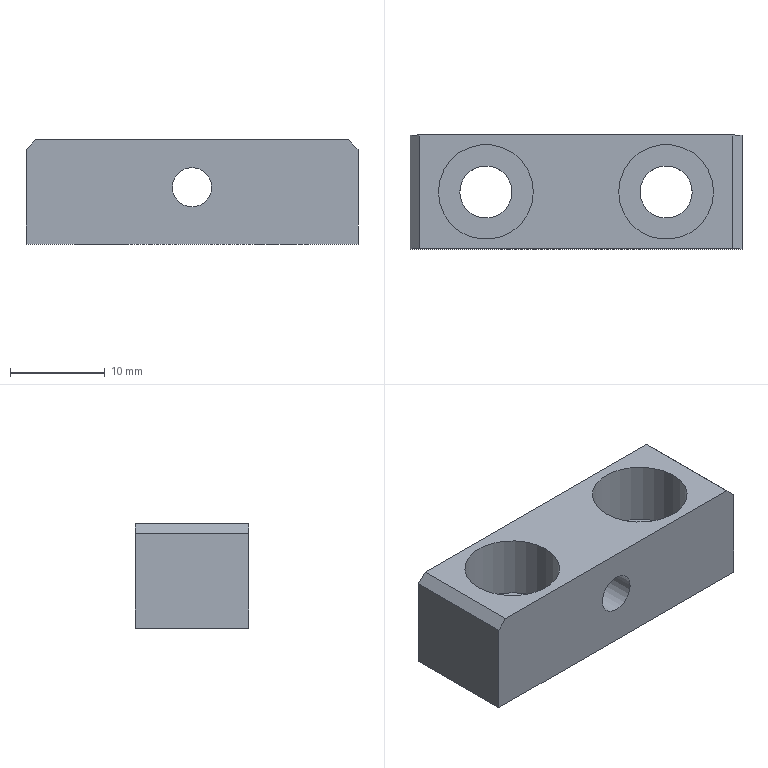Part | NX | features 5003_233_Adjusting screw block 2 | 1 solid | 15 faces | box 35 x 12 x 11 mm | volume 3190 mm3 | plane 10 | cylinder 5 | commonest cylinder face diameters 5.5 x2 10 x2 4.135 x1
STEP:
#1=CARTESIAN_POINT('',(9.775,118.5,-187.));
#2=VERTEX_POINT('',#1);
#3=CARTESIAN_POINT('',(9.775,118.5,-177.));
#4=VERTEX_POINT('',#3);
#5=CARTESIAN_POINT('',(9.775,118.5,-176.));
#6=DIRECTION('',(0.,0.,1.));
#7=VECTOR('',#6,1000.);
#8=LINE('',#5,#7);
#9=EDGE_CURVE('',#2,#4,#8,.T.);
#10=ORIENTED_EDGE('',*,*,#9,.T.);
#11=CARTESIAN_POINT('',(9.775,106.5,-177.));
#12=VERTEX_POINT('',#11);
#13=CARTESIAN_POINT('',(9.775,106.5,-177.));
#14=DIRECTION('',(0.,-1.,0.));
#15=VECTOR('',#14,1000.);
#16=LINE('',#13,#15);
#17=EDGE_CURVE('',#4,#12,#16,.T.);
#18=ORIENTED_EDGE('',*,*,#17,.T.);
#19=CARTESIAN_POINT('',(9.775,106.5,-187.));
#20=VERTEX_POINT('',#19);
#21=CARTESIAN_POINT('',(9.775,106.5,-176.));
#22=DIRECTION('',(0.,0.,1.));
#23=VECTOR('',#22,1000.);
#24=LINE('',#21,#23);
#25=EDGE_CURVE('',#20,#12,#24,.T.);
#26=ORIENTED_EDGE('',*,*,#25,.F.);
#27=CARTESIAN_POINT('',(9.775,106.5,-187.));
#28=DIRECTION('',(0.,1.,0.));
#29=VECTOR('',#28,1000.);
#30=LINE('',#27,#29);
#31=EDGE_CURVE('',#20,#2,#30,.T.);
#32=ORIENTED_EDGE('',*,*,#31,.T.);
#33=EDGE_LOOP('',(#10,#18,#26,#32));
#34=FACE_BOUND('',#33,.T.);
#35=CARTESIAN_POINT('',(9.775,106.5,-176.));
#36=DIRECTION('',(-1.,0.,0.));
#37=DIRECTION('',(0.,-1.,0.));
#38=AXIS2_PLACEMENT_3D('',#35,#36,#37);
#39=PLANE('',#38);
#40=ADVANCED_FACE('',(#34),#39,.F.);
#41=CARTESIAN_POINT('',(-22.225,112.5,-176.));
#42=VERTEX_POINT('',#41);
#43=CARTESIAN_POINT('',(-17.225,112.5,-176.));
#44=DIRECTION('',(0.,0.,1.));
#45=DIRECTION('',(-1.,0.,0.));
#46=AXIS2_PLACEMENT_3D('',#43,#44,#45);
#47=CIRCLE('',#46,5.);
#48=EDGE_CURVE('',#42,#42,#47,.T.);
#49=ORIENTED_EDGE('',*,*,#48,.F.);
#50=EDGE_LOOP('',(#49));
#51=FACE_BOUND('',#50,.T.);
#52=CARTESIAN_POINT('',(-3.225,112.5,-176.));
#53=VERTEX_POINT('',#52);
#54=CARTESIAN_POINT('',(1.775,112.5,-176.));
#55=DIRECTION('',(0.,0.,1.));
#56=DIRECTION('',(-1.,0.,0.));
#57=AXIS2_PLACEMENT_3D('',#54,#55,#56);
#58=CIRCLE('',#57,5.);
#59=EDGE_CURVE('',#53,#53,#58,.T.);
#60=ORIENTED_EDGE('',*,*,#59,.F.);
#61=EDGE_LOOP('',(#60));
#62=FACE_BOUND('',#61,.T.);
#63=CARTESIAN_POINT('',(8.775,106.5,-176.));
#64=VERTEX_POINT('',#63);
#65=CARTESIAN_POINT('',(-24.225,106.5,-176.));
#66=VERTEX_POINT('',#65);
#67=CARTESIAN_POINT('',(-25.225,106.5,-176.));
#68=DIRECTION('',(-1.,0.,0.));
#69=VECTOR('',#68,1000.);
#70=LINE('',#67,#69);
#71=EDGE_CURVE('',#64,#66,#70,.T.);
#72=ORIENTED_EDGE('',*,*,#71,.F.);
#73=CARTESIAN_POINT('',(8.775,118.5,-176.));
#74=VERTEX_POINT('',#73);
#75=CARTESIAN_POINT('',(8.775,106.5,-176.));
#76=DIRECTION('',(0.,1.,0.));
#77=VECTOR('',#76,1000.);
#78=LINE('',#75,#77);
#79=EDGE_CURVE('',#64,#74,#78,.T.);
#80=ORIENTED_EDGE('',*,*,#79,.T.);
#81=CARTESIAN_POINT('',(-24.225,118.5,-176.));
#82=VERTEX_POINT('',#81);
#83=CARTESIAN_POINT('',(-25.225,118.5,-176.));
#84=DIRECTION('',(-1.,0.,0.));
#85=VECTOR('',#84,1000.);
#86=LINE('',#83,#85);
#87=EDGE_CURVE('',#74,#82,#86,.T.);
#88=ORIENTED_EDGE('',*,*,#87,.T.);
#89=CARTESIAN_POINT('',(-24.225,106.5,-176.));
#90=DIRECTION('',(0.,-1.,0.));
#91=VECTOR('',#90,1000.);
#92=LINE('',#89,#91);
#93=EDGE_CURVE('',#82,#66,#92,.T.);
#94=ORIENTED_EDGE('',*,*,#93,.T.);
#95=EDGE_LOOP('',(#72,#80,#88,#94));
#96=FACE_BOUND('',#95,.T.);
#97=CARTESIAN_POINT('',(-25.225,106.5,-176.));
#98=DIRECTION('',(0.,0.,-1.));
#99=DIRECTION('',(1.,0.,0.));
#100=AXIS2_PLACEMENT_3D('',#97,#98,#99);
#101=PLANE('',#100);
#102=ADVANCED_FACE('',(#51,#62,#96),#101,.F.);
#103=CARTESIAN_POINT('',(-25.225,106.5,-177.));
#104=VERTEX_POINT('',#103);
#105=CARTESIAN_POINT('',(-25.225,106.5,-187.));
#106=VERTEX_POINT('',#105);
#107=CARTESIAN_POINT('',(-25.225,106.5,-176.));
#108=DIRECTION('',(0.,0.,-1.));
#109=VECTOR('',#108,1000.);
#110=LINE('',#107,#109);
#111=EDGE_CURVE('',#104,#106,#110,.T.);
#112=ORIENTED_EDGE('',*,*,#111,.F.);
#113=CARTESIAN_POINT('',(-25.225,118.5,-177.));
#114=VERTEX_POINT('',#113);
#115=CARTESIAN_POINT('',(-25.225,106.5,-177.));
#116=DIRECTION('',(0.,1.,0.));
#117=VECTOR('',#116,1000.);
#118=LINE('',#115,#117);
#119=EDGE_CURVE('',#104,#114,#118,.T.);
#120=ORIENTED_EDGE('',*,*,#119,.T.);
#121=CARTESIAN_POINT('',(-25.225,118.5,-187.));
#122=VERTEX_POINT('',#121);
#123=CARTESIAN_POINT('',(-25.225,118.5,-176.));
#124=DIRECTION('',(0.,0.,-1.));
#125=VECTOR('',#124,1000.);
#126=LINE('',#123,#125);
#127=EDGE_CURVE('',#114,#122,#126,.T.);
#128=ORIENTED_EDGE('',*,*,#127,.T.);
#129=CARTESIAN_POINT('',(-25.225,106.5,-187.));
#130=DIRECTION('',(0.,1.,0.));
#131=VECTOR('',#130,1000.);
#132=LINE('',#129,#131);
#133=EDGE_CURVE('',#106,#122,#132,.T.);
#134=ORIENTED_EDGE('',*,*,#133,.F.);
#135=EDGE_LOOP('',(#112,#120,#128,#134));
#136=FACE_BOUND('',#135,.T.);
#137=CARTESIAN_POINT('',(-25.225,106.5,-176.));
#138=DIRECTION('',(1.,0.,0.));
#139=DIRECTION('',(0.,1.,0.));
#140=AXIS2_PLACEMENT_3D('',#137,#138,#139);
#141=PLANE('',#140);
#142=ADVANCED_FACE('',(#136),#141,.F.);
#143=CARTESIAN_POINT('',(-19.975,112.5,-187.));
#144=VERTEX_POINT('',#143);
#145=CARTESIAN_POINT('',(-17.225,112.5,-187.));
#146=DIRECTION('',(0.,0.,1.));
#147=DIRECTION('',(-1.,0.,0.));
#148=AXIS2_PLACEMENT_3D('',#145,#146,#147);
#149=CIRCLE('',#148,2.75);
#150=EDGE_CURVE('',#144,#144,#149,.T.);
#151=ORIENTED_EDGE('',*,*,#150,.T.);
#152=EDGE_LOOP('',(#151));
#153=FACE_BOUND('',#152,.T.);
#154=CARTESIAN_POINT('',(-0.975,112.5,-187.));
#155=VERTEX_POINT('',#154);
#156=CARTESIAN_POINT('',(1.775,112.5,-187.));
#157=DIRECTION('',(0.,0.,1.));
#158=DIRECTION('',(-1.,0.,0.));
#159=AXIS2_PLACEMENT_3D('',#156,#157,#158);
#160=CIRCLE('',#159,2.75);
#161=EDGE_CURVE('',#155,#155,#160,.T.);
#162=ORIENTED_EDGE('',*,*,#161,.T.);
#163=EDGE_LOOP('',(#162));
#164=FACE_BOUND('',#163,.T.);
#165=CARTESIAN_POINT('',(-25.225,118.5,-187.));
#166=DIRECTION('',(1.,0.,0.));
#167=VECTOR('',#166,1000.);
#168=LINE('',#165,#167);
#169=EDGE_CURVE('',#122,#2,#168,.T.);
#170=ORIENTED_EDGE('',*,*,#169,.T.);
#171=ORIENTED_EDGE('',*,*,#31,.F.);
#172=CARTESIAN_POINT('',(-25.225,106.5,-187.));
#173=DIRECTION('',(1.,0.,0.));
#174=VECTOR('',#173,1000.);
#175=LINE('',#172,#174);
#176=EDGE_CURVE('',#106,#20,#175,.T.);
#177=ORIENTED_EDGE('',*,*,#176,.F.);
#178=ORIENTED_EDGE('',*,*,#133,.T.);
#179=EDGE_LOOP('',(#170,#171,#177,#178));
#180=FACE_BOUND('',#179,.T.);
#181=CARTESIAN_POINT('',(-25.225,106.5,-187.));
#182=DIRECTION('',(0.,0.,1.));
#183=DIRECTION('',(-1.,0.,0.));
#184=AXIS2_PLACEMENT_3D('',#181,#182,#183);
#185=PLANE('',#184);
#186=ADVANCED_FACE('',(#153,#164,#180),#185,.F.);
#187=CARTESIAN_POINT('',(-5.657,106.5,-181.));
#188=VERTEX_POINT('',#187);
#189=CARTESIAN_POINT('',(-7.725,106.5,-181.));
#190=DIRECTION('',(0.,-1.,0.));
#191=DIRECTION('',(1.,0.,0.));
#192=AXIS2_PLACEMENT_3D('',#189,#190,#191);
#193=CIRCLE('',#192,2.067);
#194=EDGE_CURVE('',#188,#188,#193,.T.);
#195=ORIENTED_EDGE('',*,*,#194,.F.);
#196=EDGE_LOOP('',(#195));
#197=FACE_BOUND('',#196,.T.);
#198=ORIENTED_EDGE('',*,*,#25,.T.);
#199=CARTESIAN_POINT('',(3.275,106.5,-170.5));
#200=DIRECTION('',(0.7071,0.,-0.7071));
#201=VECTOR('',#200,1000.);
#202=LINE('',#199,#201);
#203=EDGE_CURVE('',#12,#64,#202,.F.);
#204=ORIENTED_EDGE('',*,*,#203,.T.);
#205=ORIENTED_EDGE('',*,*,#71,.T.);
#206=CARTESIAN_POINT('',(-18.725,106.5,-170.5));
#207=DIRECTION('',(0.7071,0.,0.7071));
#208=VECTOR('',#207,1000.);
#209=LINE('',#206,#208);
#210=EDGE_CURVE('',#66,#104,#209,.F.);
#211=ORIENTED_EDGE('',*,*,#210,.T.);
#212=ORIENTED_EDGE('',*,*,#111,.T.);
#213=ORIENTED_EDGE('',*,*,#176,.T.);
#214=EDGE_LOOP('',(#198,#204,#205,#211,#212,#213));
#215=FACE_BOUND('',#214,.T.);
#216=CARTESIAN_POINT('',(-7.725,106.5,-181.5));
#217=DIRECTION('',(0.,-1.,0.));
#218=DIRECTION('',(1.,0.,0.));
#219=AXIS2_PLACEMENT_3D('',#216,#217,#218);
#220=PLANE('',#219);
#221=ADVANCED_FACE('',(#197,#215),#220,.T.);
#222=CARTESIAN_POINT('',(-5.657,118.5,-181.));
#223=VERTEX_POINT('',#222);
#224=CARTESIAN_POINT('',(-7.725,118.5,-181.));
#225=DIRECTION('',(0.,-1.,0.));
#226=DIRECTION('',(1.,0.,0.));
#227=AXIS2_PLACEMENT_3D('',#224,#225,#226);
#228=CIRCLE('',#227,2.067);
#229=EDGE_CURVE('',#223,#223,#228,.T.);
#230=ORIENTED_EDGE('',*,*,#229,.T.);
#231=EDGE_LOOP('',(#230));
#232=FACE_BOUND('',#231,.T.);
#233=ORIENTED_EDGE('',*,*,#87,.F.);
#234=CARTESIAN_POINT('',(8.775,118.5,-176.));
#235=DIRECTION('',(-0.7071,0.,0.7071));
#236=VECTOR('',#235,1000.);
#237=LINE('',#234,#236);
#238=EDGE_CURVE('',#74,#4,#237,.F.);
#239=ORIENTED_EDGE('',*,*,#238,.T.);
#240=ORIENTED_EDGE('',*,*,#9,.F.);
#241=ORIENTED_EDGE('',*,*,#169,.F.);
#242=ORIENTED_EDGE('',*,*,#127,.F.);
#243=CARTESIAN_POINT('',(-25.225,118.5,-177.));
#244=DIRECTION('',(-0.7071,0.,-0.7071));
#245=VECTOR('',#244,1000.);
#246=LINE('',#243,#245);
#247=EDGE_CURVE('',#114,#82,#246,.F.);
#248=ORIENTED_EDGE('',*,*,#247,.T.);
#249=EDGE_LOOP('',(#233,#239,#240,#241,#242,#248));
#250=FACE_BOUND('',#249,.T.);
#251=CARTESIAN_POINT('',(-7.725,118.5,-181.5));
#252=DIRECTION('',(0.,-1.,0.));
#253=DIRECTION('',(1.,0.,0.));
#254=AXIS2_PLACEMENT_3D('',#251,#252,#253);
#255=PLANE('',#254);
#256=ADVANCED_FACE('',(#232,#250),#255,.F.);
#257=ORIENTED_EDGE('',*,*,#161,.F.);
#258=EDGE_LOOP('',(#257));
#259=FACE_BOUND('',#258,.T.);
#260=CARTESIAN_POINT('',(-0.975,112.5,-182.7));
#261=VERTEX_POINT('',#260);
#262=CARTESIAN_POINT('',(1.775,112.5,-182.7));
#263=DIRECTION('',(0.,0.,1.));
#264=DIRECTION('',(-1.,0.,0.));
#265=AXIS2_PLACEMENT_3D('',#262,#263,#264);
#266=CIRCLE('',#265,2.75);
#267=EDGE_CURVE('',#261,#261,#266,.T.);
#268=ORIENTED_EDGE('',*,*,#267,.T.);
#269=EDGE_LOOP('',(#268));
#270=FACE_BOUND('',#269,.T.);
#271=CARTESIAN_POINT('',(1.775,112.5,-176.));
#272=DIRECTION('',(0.,0.,1.));
#273=DIRECTION('',(-1.,0.,0.));
#274=AXIS2_PLACEMENT_3D('',#271,#272,#273);
#275=CYLINDRICAL_SURFACE('',#274,2.75);
#276=ADVANCED_FACE('',(#259,#270),#275,.F.);
#277=ORIENTED_EDGE('',*,*,#267,.F.);
#278=EDGE_LOOP('',(#277));
#279=FACE_BOUND('',#278,.T.);
#280=CARTESIAN_POINT('',(-3.225,112.5,-182.7));
#281=VERTEX_POINT('',#280);
#282=CARTESIAN_POINT('',(1.775,112.5,-182.7));
#283=DIRECTION('',(0.,0.,1.));
#284=DIRECTION('',(-1.,0.,0.));
#285=AXIS2_PLACEMENT_3D('',#282,#283,#284);
#286=CIRCLE('',#285,5.);
#287=EDGE_CURVE('',#281,#281,#286,.T.);
#288=ORIENTED_EDGE('',*,*,#287,.T.);
#289=EDGE_LOOP('',(#288));
#290=FACE_BOUND('',#289,.T.);
#291=CARTESIAN_POINT('',(1.775,109.75,-182.7));
#292=DIRECTION('',(0.,0.,-1.));
#293=DIRECTION('',(1.,0.,0.));
#294=AXIS2_PLACEMENT_3D('',#291,#292,#293);
#295=PLANE('',#294);
#296=ADVANCED_FACE('',(#279,#290),#295,.F.);
#297=ORIENTED_EDGE('',*,*,#287,.F.);
#298=EDGE_LOOP('',(#297));
#299=FACE_BOUND('',#298,.T.);
#300=ORIENTED_EDGE('',*,*,#59,.T.);
#301=EDGE_LOOP('',(#300));
#302=FACE_BOUND('',#301,.T.);
#303=CARTESIAN_POINT('',(1.775,112.5,-176.));
#304=DIRECTION('',(0.,0.,1.));
#305=DIRECTION('',(-1.,0.,0.));
#306=AXIS2_PLACEMENT_3D('',#303,#304,#305);
#307=CYLINDRICAL_SURFACE('',#306,5.);
#308=ADVANCED_FACE('',(#299,#302),#307,.F.);
#309=ORIENTED_EDGE('',*,*,#150,.F.);
#310=EDGE_LOOP('',(#309));
#311=FACE_BOUND('',#310,.T.);
#312=CARTESIAN_POINT('',(-19.975,112.5,-182.7));
#313=VERTEX_POINT('',#312);
#314=CARTESIAN_POINT('',(-17.225,112.5,-182.7));
#315=DIRECTION('',(0.,0.,1.));
#316=DIRECTION('',(-1.,0.,0.));
#317=AXIS2_PLACEMENT_3D('',#314,#315,#316);
#318=CIRCLE('',#317,2.75);
#319=EDGE_CURVE('',#313,#313,#318,.T.);
#320=ORIENTED_EDGE('',*,*,#319,.T.);
#321=EDGE_LOOP('',(#320));
#322=FACE_BOUND('',#321,.T.);
#323=CARTESIAN_POINT('',(-17.225,112.5,-176.));
#324=DIRECTION('',(0.,0.,1.));
#325=DIRECTION('',(-1.,0.,0.));
#326=AXIS2_PLACEMENT_3D('',#323,#324,#325);
#327=CYLINDRICAL_SURFACE('',#326,2.75);
#328=ADVANCED_FACE('',(#311,#322),#327,.F.);
#329=ORIENTED_EDGE('',*,*,#319,.F.);
#330=EDGE_LOOP('',(#329));
#331=FACE_BOUND('',#330,.T.);
#332=CARTESIAN_POINT('',(-22.225,112.5,-182.7));
#333=VERTEX_POINT('',#332);
#334=CARTESIAN_POINT('',(-17.225,112.5,-182.7));
#335=DIRECTION('',(0.,0.,1.));
#336=DIRECTION('',(-1.,0.,0.));
#337=AXIS2_PLACEMENT_3D('',#334,#335,#336);
#338=CIRCLE('',#337,5.);
#339=EDGE_CURVE('',#333,#333,#338,.T.);
#340=ORIENTED_EDGE('',*,*,#339,.T.);
#341=EDGE_LOOP('',(#340));
#342=FACE_BOUND('',#341,.T.);
#343=CARTESIAN_POINT('',(-17.225,109.75,-182.7));
#344=DIRECTION('',(0.,0.,-1.));
#345=DIRECTION('',(1.,0.,0.));
#346=AXIS2_PLACEMENT_3D('',#343,#344,#345);
#347=PLANE('',#346);
#348=ADVANCED_FACE('',(#331,#342),#347,.F.);
#349=ORIENTED_EDGE('',*,*,#339,.F.);
#350=EDGE_LOOP('',(#349));
#351=FACE_BOUND('',#350,.T.);
#352=ORIENTED_EDGE('',*,*,#48,.T.);
#353=EDGE_LOOP('',(#352));
#354=FACE_BOUND('',#353,.T.);
#355=CARTESIAN_POINT('',(-17.225,112.5,-176.));
#356=DIRECTION('',(0.,0.,1.));
#357=DIRECTION('',(-1.,0.,0.));
#358=AXIS2_PLACEMENT_3D('',#355,#356,#357);
#359=CYLINDRICAL_SURFACE('',#358,5.);
#360=ADVANCED_FACE('',(#351,#354),#359,.F.);
#361=ORIENTED_EDGE('',*,*,#229,.F.);
#362=EDGE_LOOP('',(#361));
#363=FACE_BOUND('',#362,.T.);
#364=ORIENTED_EDGE('',*,*,#194,.T.);
#365=EDGE_LOOP('',(#364));
#366=FACE_BOUND('',#365,.T.);
#367=CARTESIAN_POINT('',(-7.725,106.5,-181.));
#368=DIRECTION('',(0.,-1.,0.));
#369=DIRECTION('',(1.,0.,0.));
#370=AXIS2_PLACEMENT_3D('',#367,#368,#369);
#371=CYLINDRICAL_SURFACE('',#370,2.067);
#372=ADVANCED_FACE('',(#363,#366),#371,.F.);
#373=ORIENTED_EDGE('',*,*,#203,.F.);
#374=ORIENTED_EDGE('',*,*,#17,.F.);
#375=ORIENTED_EDGE('',*,*,#238,.F.);
#376=ORIENTED_EDGE('',*,*,#79,.F.);
#377=EDGE_LOOP('',(#373,#374,#375,#376));
#378=FACE_BOUND('',#377,.T.);
#379=CARTESIAN_POINT('',(8.775,106.5,-176.));
#380=DIRECTION('',(-0.7071,0.,-0.7071));
#381=DIRECTION('',(0.,1.,0.));
#382=AXIS2_PLACEMENT_3D('',#379,#380,#381);
#383=PLANE('',#382);
#384=ADVANCED_FACE('',(#378),#383,.F.);
#385=ORIENTED_EDGE('',*,*,#210,.F.);
#386=ORIENTED_EDGE('',*,*,#93,.F.);
#387=ORIENTED_EDGE('',*,*,#247,.F.);
#388=ORIENTED_EDGE('',*,*,#119,.F.);
#389=EDGE_LOOP('',(#385,#386,#387,#388));
#390=FACE_BOUND('',#389,.T.);
#391=CARTESIAN_POINT('',(-25.225,106.5,-177.));
#392=DIRECTION('',(0.7071,0.,-0.7071));
#393=DIRECTION('',(0.,1.,0.));
#394=AXIS2_PLACEMENT_3D('',#391,#392,#393);
#395=PLANE('',#394);
#396=ADVANCED_FACE('',(#390),#395,.F.);
#397=CLOSED_SHELL('',(#40,#102,#142,#186,#221,#256,#276,#296,#308,#328,#348,#360,#372,#384,#396));
#398=MANIFOLD_SOLID_BREP('',#397);
#399=(LENGTH_UNIT()NAMED_UNIT(*)SI_UNIT(.MILLI.,.METRE.));
#400=UNCERTAINTY_MEASURE_WITH_UNIT(LENGTH_MEASURE(0.00001),#399,'','');
#401=(NAMED_UNIT(*)PLANE_ANGLE_UNIT()SI_UNIT($,.RADIAN.));
#402=(NAMED_UNIT(*)SI_UNIT($,.STERADIAN.)SOLID_ANGLE_UNIT());
#403=(GEOMETRIC_REPRESENTATION_CONTEXT(3)GLOBAL_UNCERTAINTY_ASSIGNED_CONTEXT((#400))GLOBAL_UNIT_ASSIGNED_CONTEXT((#399,#401,#402))REPRESENTATION_CONTEXT('',''));
#404=ADVANCED_BREP_SHAPE_REPRESENTATION('',(#398),#403);